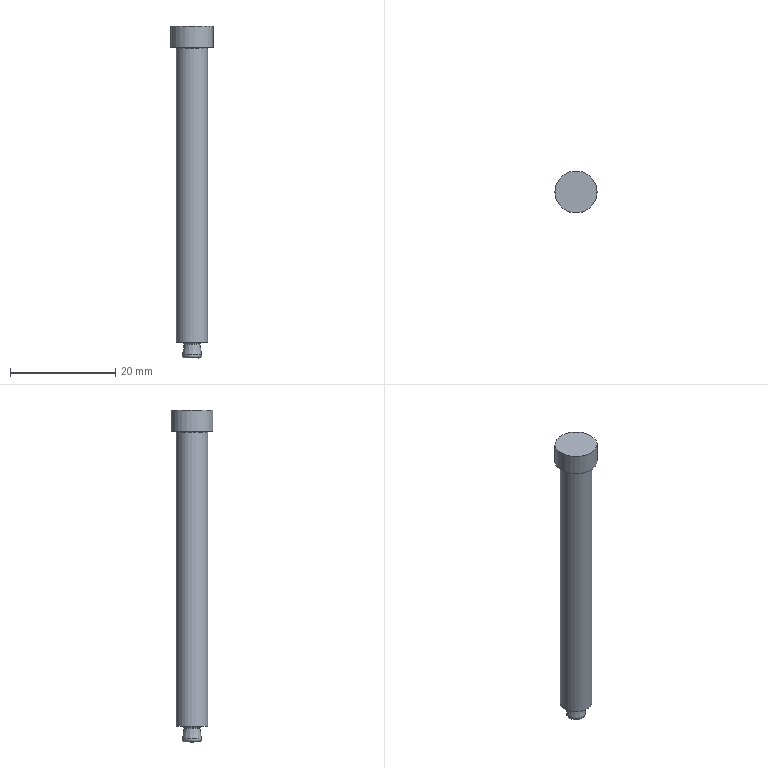Part | STEP file | 1_id530_xmt_txt | 1 solid | 11 faces | box 8 x 8 x 63 mm | volume 1811 mm3 | plane 4 | torus 3 | cylinder 2 | cone 2 | commonest cylinder face diameters 6 x1 8 x1
STEP:
#1=CARTESIAN_POINT('',(1.542,0.,103.785));
#2=VERTEX_POINT('',#1);
#3=CARTESIAN_POINT('',(0.,0.,103.785));
#4=DIRECTION('',(0.,0.,-1.));
#5=DIRECTION('',(1.,0.,0.));
#6=AXIS2_PLACEMENT_3D('',#3,#4,#5);
#7=CIRCLE('',#6,1.542);
#8=EDGE_CURVE('',#2,#2,#7,.T.);
#9=ORIENTED_EDGE('',*,*,#8,.T.);
#10=EDGE_LOOP('',(#9));
#11=FACE_BOUND('',#10,.T.);
#12=CARTESIAN_POINT('',(1.514,0.,103.606));
#13=VERTEX_POINT('',#12);
#14=CARTESIAN_POINT('',(0.,0.,103.606));
#15=DIRECTION('',(0.,0.,1.));
#16=DIRECTION('',(1.,0.,0.));
#17=AXIS2_PLACEMENT_3D('',#14,#15,#16);
#18=CIRCLE('',#17,1.514);
#19=EDGE_CURVE('',#13,#13,#18,.T.);
#20=ORIENTED_EDGE('',*,*,#19,.T.);
#21=EDGE_LOOP('',(#20));
#22=FACE_BOUND('',#21,.T.);
#23=CARTESIAN_POINT('',(0.,0.,103.65));
#24=DIRECTION('',(0.,0.,-1.));
#25=DIRECTION('',(-1.,0.,0.));
#26=AXIS2_PLACEMENT_3D('',#23,#24,#25);
#27=TOROIDAL_SURFACE('',#26,1.811,0.3);
#28=ADVANCED_FACE('',(#11,#22),#27,.F.);
#29=CARTESIAN_POINT('',(1.32,0.,101.));
#30=VERTEX_POINT('',#29);
#31=CARTESIAN_POINT('',(0.,0.,101.));
#32=DIRECTION('',(0.,0.,1.));
#33=DIRECTION('',(1.,0.,0.));
#34=AXIS2_PLACEMENT_3D('',#31,#32,#33);
#35=CIRCLE('',#34,1.32);
#36=EDGE_CURVE('',#30,#30,#35,.T.);
#37=ORIENTED_EDGE('',*,*,#36,.T.);
#38=EDGE_LOOP('',(#37));
#39=FACE_BOUND('',#38,.T.);
#40=CARTESIAN_POINT('',(1.815,0.,101.573));
#41=VERTEX_POINT('',#40);
#42=CARTESIAN_POINT('',(0.,0.,101.573));
#43=DIRECTION('',(0.,0.,-1.));
#44=DIRECTION('',(1.,0.,0.));
#45=AXIS2_PLACEMENT_3D('',#42,#43,#44);
#46=CIRCLE('',#45,1.815);
#47=EDGE_CURVE('',#41,#41,#46,.T.);
#48=ORIENTED_EDGE('',*,*,#47,.T.);
#49=EDGE_LOOP('',(#48));
#50=FACE_BOUND('',#49,.T.);
#51=CARTESIAN_POINT('',(0.,0.,101.5));
#52=DIRECTION('',(0.,0.,-1.));
#53=DIRECTION('',(1.,0.,0.));
#54=AXIS2_PLACEMENT_3D('',#51,#52,#53);
#55=TOROIDAL_SURFACE('',#54,1.32,0.5);
#56=ADVANCED_FACE('',(#39,#50),#55,.T.);
#57=CARTESIAN_POINT('',(-4.,0.,164.));
#58=VERTEX_POINT('',#57);
#59=CARTESIAN_POINT('',(0.,0.,164.));
#60=DIRECTION('',(0.,0.,1.));
#61=DIRECTION('',(-1.,0.,0.));
#62=AXIS2_PLACEMENT_3D('',#59,#60,#61);
#63=CIRCLE('',#62,4.);
#64=EDGE_CURVE('',#58,#58,#63,.T.);
#65=ORIENTED_EDGE('',*,*,#64,.F.);
#66=EDGE_LOOP('',(#65));
#67=FACE_BOUND('',#66,.T.);
#68=CARTESIAN_POINT('',(-4.,0.,160.));
#69=VERTEX_POINT('',#68);
#70=CARTESIAN_POINT('',(0.,0.,160.));
#71=DIRECTION('',(0.,0.,-1.));
#72=DIRECTION('',(-1.,0.,0.));
#73=AXIS2_PLACEMENT_3D('',#70,#71,#72);
#74=CIRCLE('',#73,4.);
#75=EDGE_CURVE('',#69,#69,#74,.T.);
#76=ORIENTED_EDGE('',*,*,#75,.F.);
#77=EDGE_LOOP('',(#76));
#78=FACE_BOUND('',#77,.T.);
#79=CARTESIAN_POINT('',(0.,0.,162.));
#80=DIRECTION('',(0.,0.,-1.));
#81=DIRECTION('',(1.,0.,0.));
#82=AXIS2_PLACEMENT_3D('',#79,#80,#81);
#83=CYLINDRICAL_SURFACE('',#82,4.);
#84=ADVANCED_FACE('',(#67,#78),#83,.T.);
#85=CARTESIAN_POINT('',(3.,0.,159.7));
#86=VERTEX_POINT('',#85);
#87=CARTESIAN_POINT('',(0.,0.,159.7));
#88=DIRECTION('',(0.,0.,1.));
#89=DIRECTION('',(1.,0.,0.));
#90=AXIS2_PLACEMENT_3D('',#87,#88,#89);
#91=CIRCLE('',#90,3.);
#92=EDGE_CURVE('',#86,#86,#91,.T.);
#93=ORIENTED_EDGE('',*,*,#92,.F.);
#94=EDGE_LOOP('',(#93));
#95=FACE_BOUND('',#94,.T.);
#96=CARTESIAN_POINT('',(-3.,0.,104.));
#97=VERTEX_POINT('',#96);
#98=CARTESIAN_POINT('',(0.,0.,104.));
#99=DIRECTION('',(0.,0.,-1.));
#100=DIRECTION('',(-1.,0.,0.));
#101=AXIS2_PLACEMENT_3D('',#98,#99,#100);
#102=CIRCLE('',#101,3.);
#103=EDGE_CURVE('',#97,#97,#102,.T.);
#104=ORIENTED_EDGE('',*,*,#103,.F.);
#105=EDGE_LOOP('',(#104));
#106=FACE_BOUND('',#105,.T.);
#107=CARTESIAN_POINT('',(0.,0.,132.));
#108=DIRECTION('',(0.,0.,-1.));
#109=DIRECTION('',(1.,0.,0.));
#110=AXIS2_PLACEMENT_3D('',#107,#108,#109);
#111=CYLINDRICAL_SURFACE('',#110,3.);
#112=ADVANCED_FACE('',(#95,#106),#111,.T.);
#113=ORIENTED_EDGE('',*,*,#92,.T.);
#114=EDGE_LOOP('',(#113));
#115=FACE_BOUND('',#114,.T.);
#116=CARTESIAN_POINT('',(3.3,0.,160.));
#117=VERTEX_POINT('',#116);
#118=CARTESIAN_POINT('',(0.,0.,160.));
#119=DIRECTION('',(0.,0.,-1.));
#120=DIRECTION('',(1.,0.,0.));
#121=AXIS2_PLACEMENT_3D('',#118,#119,#120);
#122=CIRCLE('',#121,3.3);
#123=EDGE_CURVE('',#117,#117,#122,.T.);
#124=ORIENTED_EDGE('',*,*,#123,.T.);
#125=EDGE_LOOP('',(#124));
#126=FACE_BOUND('',#125,.T.);
#127=CARTESIAN_POINT('',(0.,0.,159.7));
#128=DIRECTION('',(0.,0.,1.));
#129=DIRECTION('',(-1.,0.,0.));
#130=AXIS2_PLACEMENT_3D('',#127,#128,#129);
#131=TOROIDAL_SURFACE('',#130,3.3,0.3);
#132=ADVANCED_FACE('',(#115,#126),#131,.F.);
#133=CARTESIAN_POINT('',(-1.65,0.,104.));
#134=VERTEX_POINT('',#133);
#135=CARTESIAN_POINT('',(0.,0.,104.));
#136=DIRECTION('',(0.,0.,1.));
#137=DIRECTION('',(-1.,0.,0.));
#138=AXIS2_PLACEMENT_3D('',#135,#136,#137);
#139=CIRCLE('',#138,1.65);
#140=EDGE_CURVE('',#134,#134,#139,.T.);
#141=ORIENTED_EDGE('',*,*,#140,.F.);
#142=EDGE_LOOP('',(#141));
#143=FACE_BOUND('',#142,.T.);
#144=ORIENTED_EDGE('',*,*,#8,.F.);
#145=EDGE_LOOP('',(#144));
#146=FACE_BOUND('',#145,.T.);
#147=CARTESIAN_POINT('',(0.,0.,103.85));
#148=DIRECTION('',(0.,0.,1.));
#149=DIRECTION('',(1.,0.,0.));
#150=AXIS2_PLACEMENT_3D('',#147,#148,#149);
#151=CONICAL_SURFACE('',#150,1.575,26.565);
#152=ADVANCED_FACE('',(#143,#146),#151,.T.);
#153=ORIENTED_EDGE('',*,*,#19,.F.);
#154=EDGE_LOOP('',(#153));
#155=FACE_BOUND('',#154,.T.);
#156=ORIENTED_EDGE('',*,*,#47,.F.);
#157=EDGE_LOOP('',(#156));
#158=FACE_BOUND('',#157,.T.);
#159=CARTESIAN_POINT('',(0.,0.,102.35));
#160=DIRECTION('',(0.,0.,-1.));
#161=DIRECTION('',(1.,0.,0.));
#162=AXIS2_PLACEMENT_3D('',#159,#160,#161);
#163=CONICAL_SURFACE('',#162,1.7,8.427);
#164=ADVANCED_FACE('',(#155,#158),#163,.T.);
#165=ORIENTED_EDGE('',*,*,#36,.F.);
#166=EDGE_LOOP('',(#165));
#167=FACE_OUTER_BOUND('',#166,.T.);
#168=CARTESIAN_POINT('',(0.,0.,101.));
#169=DIRECTION('',(0.,0.,-1.));
#170=DIRECTION('',(1.,0.,0.));
#171=AXIS2_PLACEMENT_3D('',#168,#169,#170);
#172=PLANE('',#171);
#173=ADVANCED_FACE('',(#167),#172,.T.);
#174=ORIENTED_EDGE('',*,*,#75,.T.);
#175=EDGE_LOOP('',(#174));
#176=FACE_BOUND('',#175,.T.);
#177=ORIENTED_EDGE('',*,*,#123,.F.);
#178=EDGE_LOOP('',(#177));
#179=FACE_BOUND('',#178,.T.);
#180=CARTESIAN_POINT('',(0.,0.,160.));
#181=DIRECTION('',(0.,0.,-1.));
#182=DIRECTION('',(1.,0.,0.));
#183=AXIS2_PLACEMENT_3D('',#180,#181,#182);
#184=PLANE('',#183);
#185=ADVANCED_FACE('',(#176,#179),#184,.T.);
#186=ORIENTED_EDGE('',*,*,#140,.T.);
#187=EDGE_LOOP('',(#186));
#188=FACE_BOUND('',#187,.T.);
#189=ORIENTED_EDGE('',*,*,#103,.T.);
#190=EDGE_LOOP('',(#189));
#191=FACE_BOUND('',#190,.T.);
#192=CARTESIAN_POINT('',(0.,0.,104.));
#193=DIRECTION('',(0.,0.,-1.));
#194=DIRECTION('',(1.,0.,0.));
#195=AXIS2_PLACEMENT_3D('',#192,#193,#194);
#196=PLANE('',#195);
#197=ADVANCED_FACE('',(#188,#191),#196,.T.);
#198=ORIENTED_EDGE('',*,*,#64,.T.);
#199=EDGE_LOOP('',(#198));
#200=FACE_OUTER_BOUND('',#199,.T.);
#201=CARTESIAN_POINT('',(0.,0.,164.));
#202=DIRECTION('',(0.,0.,1.));
#203=DIRECTION('',(-1.,0.,0.));
#204=AXIS2_PLACEMENT_3D('',#201,#202,#203);
#205=PLANE('',#204);
#206=ADVANCED_FACE('',(#200),#205,.T.);
#207=CLOSED_SHELL('',(#28,#56,#84,#112,#132,#152,#164,#173,#185,#197,#206));
#208=MANIFOLD_SOLID_BREP('',#207);
#209=(LENGTH_UNIT()NAMED_UNIT(*)SI_UNIT(.MILLI.,.METRE.));
#210=UNCERTAINTY_MEASURE_WITH_UNIT(LENGTH_MEASURE(0.00002),#209,'','');
#211=(NAMED_UNIT(*)PLANE_ANGLE_UNIT()SI_UNIT($,.RADIAN.));
#212=PLANE_ANGLE_MEASURE_WITH_UNIT(PLANE_ANGLE_MEASURE(0.01745),#211);
#213=DIMENSIONAL_EXPONENTS(0.,0.,0.,0.,0.,0.,0.);
#214=(CONVERSION_BASED_UNIT('DEGREE',#212)NAMED_UNIT(#213)PLANE_ANGLE_UNIT());
#215=(NAMED_UNIT(*)SI_UNIT($,.STERADIAN.)SOLID_ANGLE_UNIT());
#216=(GEOMETRIC_REPRESENTATION_CONTEXT(3)GLOBAL_UNCERTAINTY_ASSIGNED_CONTEXT((#210))GLOBAL_UNIT_ASSIGNED_CONTEXT((#209,#214,#215))REPRESENTATION_CONTEXT('',''));
#217=ADVANCED_BREP_SHAPE_REPRESENTATION('',(#208),#216);